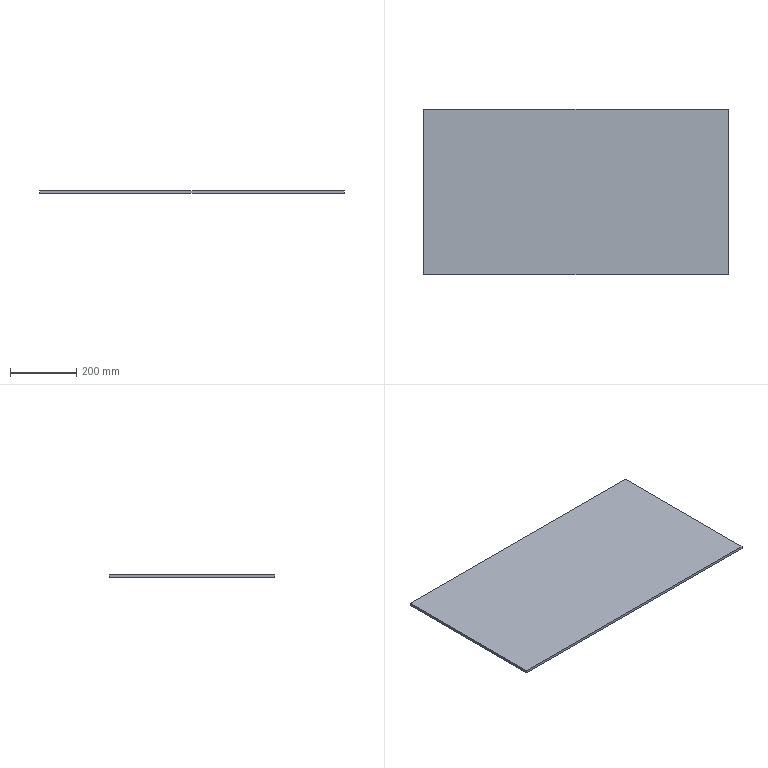Part | SolidWorks | features Extrusion 1 | 1 solid | 6 faces | box 920 x 500 x 8 mm | volume 3680000 mm3 | plane 6
STEP:
#1=CARTESIAN_POINT('',(-460.,250.,0.));
#2=VERTEX_POINT('',#1);
#3=CARTESIAN_POINT('',(-460.,-250.,0.));
#4=VERTEX_POINT('',#3);
#5=CARTESIAN_POINT('',(-460.,250.,0.));
#6=DIRECTION('',(0.,-1.,0.));
#7=VECTOR('',#6,1000.);
#8=LINE('',#5,#7);
#9=EDGE_CURVE('',#2,#4,#8,.T.);
#10=ORIENTED_EDGE('',*,*,#9,.T.);
#11=CARTESIAN_POINT('',(-460.,-250.,8.));
#12=VERTEX_POINT('',#11);
#13=CARTESIAN_POINT('',(-460.,-250.,8.));
#14=DIRECTION('',(0.,0.,-1.));
#15=VECTOR('',#14,1000.);
#16=LINE('',#13,#15);
#17=EDGE_CURVE('',#12,#4,#16,.T.);
#18=ORIENTED_EDGE('',*,*,#17,.F.);
#19=CARTESIAN_POINT('',(-460.,250.,8.));
#20=VERTEX_POINT('',#19);
#21=CARTESIAN_POINT('',(-460.,250.,8.));
#22=DIRECTION('',(0.,-1.,0.));
#23=VECTOR('',#22,1000.);
#24=LINE('',#21,#23);
#25=EDGE_CURVE('',#20,#12,#24,.T.);
#26=ORIENTED_EDGE('',*,*,#25,.F.);
#27=CARTESIAN_POINT('',(-460.,250.,8.));
#28=DIRECTION('',(0.,0.,-1.));
#29=VECTOR('',#28,1000.);
#30=LINE('',#27,#29);
#31=EDGE_CURVE('',#20,#2,#30,.T.);
#32=ORIENTED_EDGE('',*,*,#31,.T.);
#33=EDGE_LOOP('',(#10,#18,#26,#32));
#34=FACE_OUTER_BOUND('',#33,.T.);
#35=CARTESIAN_POINT('',(-460.,250.,8.));
#36=DIRECTION('',(1.,0.,0.));
#37=DIRECTION('',(0.,1.,0.));
#38=AXIS2_PLACEMENT_3D('',#35,#36,#37);
#39=PLANE('',#38);
#40=ADVANCED_FACE('',(#34),#39,.F.);
#41=CARTESIAN_POINT('',(460.,-250.,0.));
#42=VERTEX_POINT('',#41);
#43=CARTESIAN_POINT('',(460.,-250.,0.));
#44=DIRECTION('',(1.,0.,0.));
#45=VECTOR('',#44,1000.);
#46=LINE('',#43,#45);
#47=EDGE_CURVE('',#4,#42,#46,.T.);
#48=ORIENTED_EDGE('',*,*,#47,.T.);
#49=CARTESIAN_POINT('',(460.,-250.,8.));
#50=VERTEX_POINT('',#49);
#51=CARTESIAN_POINT('',(460.,-250.,8.));
#52=DIRECTION('',(0.,0.,-1.));
#53=VECTOR('',#52,1000.);
#54=LINE('',#51,#53);
#55=EDGE_CURVE('',#50,#42,#54,.T.);
#56=ORIENTED_EDGE('',*,*,#55,.F.);
#57=CARTESIAN_POINT('',(460.,-250.,8.));
#58=DIRECTION('',(1.,0.,0.));
#59=VECTOR('',#58,1000.);
#60=LINE('',#57,#59);
#61=EDGE_CURVE('',#12,#50,#60,.T.);
#62=ORIENTED_EDGE('',*,*,#61,.F.);
#63=ORIENTED_EDGE('',*,*,#17,.T.);
#64=EDGE_LOOP('',(#48,#56,#62,#63));
#65=FACE_OUTER_BOUND('',#64,.T.);
#66=CARTESIAN_POINT('',(460.,-250.,8.));
#67=DIRECTION('',(0.,1.,0.));
#68=DIRECTION('',(-1.,0.,0.));
#69=AXIS2_PLACEMENT_3D('',#66,#67,#68);
#70=PLANE('',#69);
#71=ADVANCED_FACE('',(#65),#70,.F.);
#72=CARTESIAN_POINT('',(460.,250.,0.));
#73=VERTEX_POINT('',#72);
#74=CARTESIAN_POINT('',(460.,250.,0.));
#75=DIRECTION('',(0.,1.,0.));
#76=VECTOR('',#75,1000.);
#77=LINE('',#74,#76);
#78=EDGE_CURVE('',#42,#73,#77,.T.);
#79=ORIENTED_EDGE('',*,*,#78,.T.);
#80=CARTESIAN_POINT('',(460.,250.,8.));
#81=VERTEX_POINT('',#80);
#82=CARTESIAN_POINT('',(460.,250.,8.));
#83=DIRECTION('',(0.,0.,-1.));
#84=VECTOR('',#83,1000.);
#85=LINE('',#82,#84);
#86=EDGE_CURVE('',#81,#73,#85,.T.);
#87=ORIENTED_EDGE('',*,*,#86,.F.);
#88=CARTESIAN_POINT('',(460.,250.,8.));
#89=DIRECTION('',(0.,1.,0.));
#90=VECTOR('',#89,1000.);
#91=LINE('',#88,#90);
#92=EDGE_CURVE('',#50,#81,#91,.T.);
#93=ORIENTED_EDGE('',*,*,#92,.F.);
#94=ORIENTED_EDGE('',*,*,#55,.T.);
#95=EDGE_LOOP('',(#79,#87,#93,#94));
#96=FACE_OUTER_BOUND('',#95,.T.);
#97=CARTESIAN_POINT('',(460.,250.,8.));
#98=DIRECTION('',(-1.,0.,0.));
#99=DIRECTION('',(0.,-1.,0.));
#100=AXIS2_PLACEMENT_3D('',#97,#98,#99);
#101=PLANE('',#100);
#102=ADVANCED_FACE('',(#96),#101,.F.);
#103=CARTESIAN_POINT('',(460.,250.,0.));
#104=DIRECTION('',(-1.,0.,0.));
#105=VECTOR('',#104,1000.);
#106=LINE('',#103,#105);
#107=EDGE_CURVE('',#73,#2,#106,.T.);
#108=ORIENTED_EDGE('',*,*,#107,.T.);
#109=ORIENTED_EDGE('',*,*,#31,.F.);
#110=CARTESIAN_POINT('',(460.,250.,8.));
#111=DIRECTION('',(-1.,0.,0.));
#112=VECTOR('',#111,1000.);
#113=LINE('',#110,#112);
#114=EDGE_CURVE('',#81,#20,#113,.T.);
#115=ORIENTED_EDGE('',*,*,#114,.F.);
#116=ORIENTED_EDGE('',*,*,#86,.T.);
#117=EDGE_LOOP('',(#108,#109,#115,#116));
#118=FACE_OUTER_BOUND('',#117,.T.);
#119=CARTESIAN_POINT('',(460.,250.,8.));
#120=DIRECTION('',(0.,-1.,0.));
#121=DIRECTION('',(1.,0.,0.));
#122=AXIS2_PLACEMENT_3D('',#119,#120,#121);
#123=PLANE('',#122);
#124=ADVANCED_FACE('',(#118),#123,.F.);
#125=ORIENTED_EDGE('',*,*,#25,.T.);
#126=ORIENTED_EDGE('',*,*,#61,.T.);
#127=ORIENTED_EDGE('',*,*,#92,.T.);
#128=ORIENTED_EDGE('',*,*,#114,.T.);
#129=EDGE_LOOP('',(#125,#126,#127,#128));
#130=FACE_OUTER_BOUND('',#129,.T.);
#131=CARTESIAN_POINT('',(0.,0.,8.));
#132=DIRECTION('',(0.,0.,-1.));
#133=DIRECTION('',(-1.,0.,0.));
#134=AXIS2_PLACEMENT_3D('',#131,#132,#133);
#135=PLANE('',#134);
#136=ADVANCED_FACE('',(#130),#135,.F.);
#137=ORIENTED_EDGE('',*,*,#9,.F.);
#138=ORIENTED_EDGE('',*,*,#107,.F.);
#139=ORIENTED_EDGE('',*,*,#78,.F.);
#140=ORIENTED_EDGE('',*,*,#47,.F.);
#141=EDGE_LOOP('',(#137,#138,#139,#140));
#142=FACE_OUTER_BOUND('',#141,.T.);
#143=CARTESIAN_POINT('',(0.,0.,0.));
#144=DIRECTION('',(0.,0.,-1.));
#145=DIRECTION('',(-1.,0.,0.));
#146=AXIS2_PLACEMENT_3D('',#143,#144,#145);
#147=PLANE('',#146);
#148=ADVANCED_FACE('',(#142),#147,.T.);
#149=CLOSED_SHELL('',(#40,#71,#102,#124,#136,#148));
#150=MANIFOLD_SOLID_BREP('',#149);
#151=CARTESIAN_POINT('',(0.,0.,0.));
#152=DIRECTION('',(0.,0.,1.));
#153=DIRECTION('',(1.,0.,0.));
#154=AXIS2_PLACEMENT_3D('',#151,#152,#153);
#155=(LENGTH_UNIT()NAMED_UNIT(*)SI_UNIT(.MILLI.,.METRE.));
#156=UNCERTAINTY_MEASURE_WITH_UNIT(LENGTH_MEASURE(0.00001),#155,'','');
#157=(NAMED_UNIT(*)PLANE_ANGLE_UNIT()SI_UNIT($,.RADIAN.));
#158=(NAMED_UNIT(*)SI_UNIT($,.STERADIAN.)SOLID_ANGLE_UNIT());
#159=(GEOMETRIC_REPRESENTATION_CONTEXT(3)GLOBAL_UNCERTAINTY_ASSIGNED_CONTEXT((#156))GLOBAL_UNIT_ASSIGNED_CONTEXT((#155,#157,#158))REPRESENTATION_CONTEXT('',''));
#160=ADVANCED_BREP_SHAPE_REPRESENTATION('',(#150,#154),#159);